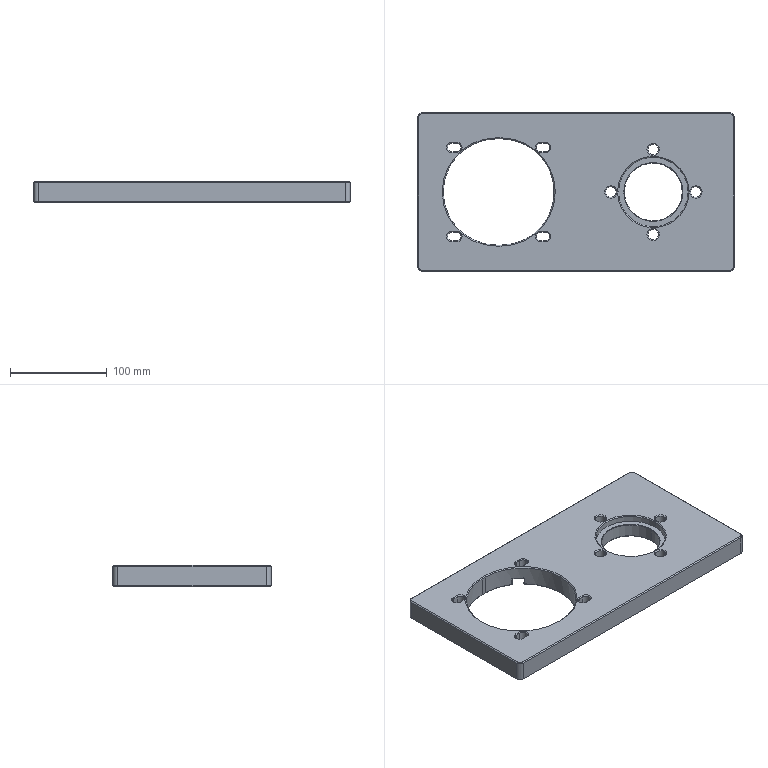NC program | NX | posted with a generic post | part box 328 x 164 x 22 mm
Lines 1 to 575 of 34171:
N10 G17 G21 G94 G90
(DRILLING , TOOL : ZXZ)
N12 T01 M6
N14 G54
N16 G17 G0 G90 X80. Y44. S5000 M3
N18 G43 Z30. H1
N20 G94 G81 G98 Z-1. F250. R3.
N22 Y0.
N24 X36.
N26 X80. Y-44.
N28 X124. Y0.
N30 G80
N32 G0 X124. Y0. Z30.
(DRILLING_COPY , TOOL : ZXZ)
N34 X-31.538 Y45.962
N36 G81 Z-1. F250. R3.
N38 X-123.462
N40 Y-45.962
N42 X-31.538
N44 G80
N46 G0 X-31.538 Y-45.962 Z30.
N48 M5
(DRILLING_COPY_COPY , TOOL : 11.0ZT)
N50 T11 M6
N52 G54
N54 G17 G0 G90 X80. Y44. S1200 M3
N56 G43 Z30. H11
N58 G94 G83 G98 Z-25.305 F250. Q2. R3.
N60 Y0.
N62 X36.
N64 X80. Y-44.
N66 X124. Y0.
N68 G80
N70 G0 X124. Y0. Z30.
N72 M5
(DRILLING_COPY_COPY_1 , TOOL : 6.8ZT)
N74 T16 M6
N76 G54
N78 G17 G0 G90 X-31.538 Y45.962 S2000 M3
N80 G43 Z30. H16
N82 G94 G83 G98 Z-24.043 F250. Q2. R3.
N84 X-123.462
N86 Y-45.962
N88 X-31.538
N90 G80
N92 G0 X-31.538 Y-45.962 Z30.
N94 M5
(HOLE_MILLING_COPY , TOOL : D26)
N96 T02 M6
N98 G54
N100 G17 G0 G90 X80. Y0. S1700 M3
N102 G43 Z30. H2
N104 Z0.5
N106 G94 G3 X85.713 Y-5.713 R5.712 F1000.
N108 X91.425 Y0. R5.712
N110 X91.425 Y0. Z0.2 I-11.425 J0. F2000.
N112 X91.425 Y0. Z-0.1 I-11.425 J0.
N114 X91.425 Y0. Z-0.4 I-11.425 J0.
N116 X91.425 Y0. Z-0.7 I-11.425 J0.
N118 X91.425 Y0. Z-1. I-11.425 J0.
N120 X91.425 Y0. Z-1.3 I-11.425 J0.
N122 X91.425 Y0. Z-1.6 I-11.425 J0.
N124 X91.425 Y0. Z-1.9 I-11.425 J0.
N126 X91.425 Y0. Z-2.2 I-11.425 J0.
N128 X91.425 Y0. Z-2.5 I-11.425 J0.
N130 X91.425 Y0. Z-2.8 I-11.425 J0.
N132 X91.425 Y0. Z-3.1 I-11.425 J0.
N134 X91.425 Y0. Z-3.4 I-11.425 J0.
N136 X91.425 Y0. Z-3.7 I-11.425 J0.
N138 X91.425 Y0. Z-4. I-11.425 J0.
N140 X91.425 Y0. Z-4.3 I-11.425 J0.
N142 X91.425 Y0. Z-4.6 I-11.425 J0.
N144 X91.425 Y0. Z-4.9 I-11.425 J0.
N146 X91.425 Y0. Z-5.2 I-11.425 J0.
N148 X91.425 Y0. Z-5.5 I-11.425 J0.
N150 X91.425 Y0. Z-5.8 I-11.425 J0.
N152 X91.425 Y0. Z-6.1 I-11.425 J0.
N154 X91.425 Y0. Z-6.4 I-11.425 J0.
N156 X91.425 Y0. Z-6.7 I-11.425 J0.
N158 X91.425 Y0. Z-7. I-11.425 J0.
N160 X80. Y11.425 R11.425
N162 X91.425 Y0. R-11.425
N164 X85.713 Y5.713 R5.712
N166 X80. Y0. R5.712
N168 G0 Z0.5
N170 G3 X91.425 Y-11.425 R11.425 F1000.
N172 X102.85 Y0. R11.425
N174 X102.85 Y0. Z0.2 I-22.85 J0. F2000.
N176 X102.85 Y0. Z-0.1 I-22.85 J0.
N178 X102.85 Y0. Z-0.4 I-22.85 J0.
N180 X102.85 Y0. Z-0.7 I-22.85 J0.
N182 X102.85 Y0. Z-1. I-22.85 J0.
N184 X102.85 Y0. Z-1.3 I-22.85 J0.
N186 X102.85 Y0. Z-1.6 I-22.85 J0.
N188 X102.85 Y0. Z-1.9 I-22.85 J0.
N190 X102.85 Y0. Z-2.2 I-22.85 J0.
N192 X102.85 Y0. Z-2.5 I-22.85 J0.
N194 X102.85 Y0. Z-2.8 I-22.85 J0.
N196 X102.85 Y0. Z-3.1 I-22.85 J0.
N198 X102.85 Y0. Z-3.4 I-22.85 J0.
N200 X102.85 Y0. Z-3.7 I-22.85 J0.
N202 X102.85 Y0. Z-4. I-22.85 J0.
N204 X102.85 Y0. Z-4.3 I-22.85 J0.
N206 X102.85 Y0. Z-4.6 I-22.85 J0.
N208 X102.85 Y0. Z-4.9 I-22.85 J0.
N210 X102.85 Y0. Z-5.2 I-22.85 J0.
N212 X102.85 Y0. Z-5.5 I-22.85 J0.
N214 X102.85 Y0. Z-5.8 I-22.85 J0.
N216 X102.85 Y0. Z-6.1 I-22.85 J0.
N218 X102.85 Y0. Z-6.4 I-22.85 J0.
N220 X102.85 Y0. Z-6.7 I-22.85 J0.
N222 X102.85 Y0. Z-7. I-22.85 J0.
N224 X80. Y22.85 R22.85
N226 X102.85 Y0. R-22.85
N228 X91.425 Y11.425 R11.425
N230 X80. Y0. R11.425
N232 G0 Z30.
(HOLE_MILLING_COPY_COPY , TOOL : D26)
N234 Z-6.5
N236 G3 X84.213 Y-4.213 R4.212 F1000.
N238 X88.425 Y0. R4.212
N240 X88.425 Y0. Z-6.8 I-8.425 J0. F2000.
N242 X88.425 Y0. Z-7.1 I-8.425 J0.
N244 X88.425 Y0. Z-7.4 I-8.425 J0.
N246 X88.425 Y0. Z-7.7 I-8.425 J0.
N248 X88.425 Y0. Z-8. I-8.425 J0.
N250 X88.425 Y0. Z-8.3 I-8.425 J0.
N252 X88.425 Y0. Z-8.6 I-8.425 J0.
N254 X88.425 Y0. Z-8.9 I-8.425 J0.
N256 X88.425 Y0. Z-9.2 I-8.425 J0.
N258 X88.425 Y0. Z-9.5 I-8.425 J0.
N260 X88.425 Y0. Z-9.8 I-8.425 J0.
N262 X88.425 Y0. Z-10.1 I-8.425 J0.
N264 X88.425 Y0. Z-10.4 I-8.425 J0.
N266 X88.425 Y0. Z-10.7 I-8.425 J0.
N268 X88.425 Y0. Z-11. I-8.425 J0.
N270 X88.425 Y0. Z-11.3 I-8.425 J0.
N272 X88.425 Y0. Z-11.6 I-8.425 J0.
N274 X88.425 Y0. Z-11.9 I-8.425 J0.
N276 X88.425 Y0. Z-12.2 I-8.425 J0.
N278 X88.425 Y0. Z-12.5 I-8.425 J0.
N280 X88.425 Y0. Z-12.8 I-8.425 J0.
N282 X88.425 Y0. Z-13.1 I-8.425 J0.
N284 X88.425 Y0. Z-13.4 I-8.425 J0.
N286 X88.425 Y0. Z-13.7 I-8.425 J0.
N288 X88.425 Y0. Z-14. I-8.425 J0.
N290 X88.425 Y0. Z-14.3 I-8.425 J0.
N292 X88.425 Y0. Z-14.6 I-8.425 J0.
N294 X88.425 Y0. Z-14.9 I-8.425 J0.
N296 X88.425 Y0. Z-15.2 I-8.425 J0.
N298 X88.425 Y0. Z-15.5 I-8.425 J0.
N300 X88.425 Y0. Z-15.8 I-8.425 J0.
N302 X88.425 Y0. Z-16.1 I-8.425 J0.
N304 X88.425 Y0. Z-16.4 I-8.425 J0.
N306 X88.425 Y0. Z-16.7 I-8.425 J0.
N308 X88.425 Y0. Z-17. I-8.425 J0.
N310 X88.425 Y0. Z-17.3 I-8.425 J0.
N312 X88.425 Y0. Z-17.6 I-8.425 J0.
N314 X88.425 Y0. Z-17.9 I-8.425 J0.
N316 X88.425 Y0. Z-18.2 I-8.425 J0.
N318 X88.425 Y0. Z-18.5 I-8.425 J0.
N320 X88.425 Y0. Z-18.8 I-8.425 J0.
N322 X88.425 Y0. Z-19.1 I-8.425 J0.
N324 X88.425 Y0. Z-19.4 I-8.425 J0.
N326 X88.425 Y0. Z-19.7 I-8.425 J0.
N328 X88.425 Y0. Z-20. I-8.425 J0.
N330 X88.425 Y0. Z-20.3 I-8.425 J0.
N332 X88.425 Y0. Z-20.6 I-8.425 J0.
N334 X88.425 Y0. Z-20.9 I-8.425 J0.
N336 X88.425 Y0. Z-21.2 I-8.425 J0.
N338 X88.425 Y0. Z-21.5 I-8.425 J0.
N340 X88.425 Y0. Z-21.8 I-8.425 J0.
N342 X88.425 Y0. Z-22.1 I-8.425 J0.
N344 X88.425 Y0. Z-22.4 I-8.425 J0.
N346 X88.425 Y0. Z-22.7 I-8.425 J0.
N348 X75.788 Y7.296 Z-22.8 R8.425
N350 X72.704 Y-4.213 R8.425
N352 X75.788 Y7.296 R-8.425
N354 X74.246 Y1.542 R4.212
N356 X80. Y0. R4.212
N358 G0 Z-6.5
N360 G3 X88.425 Y-8.425 R8.425 F1000.
N362 X96.85 Y0. R8.425
N364 X96.85 Y0. Z-6.8 I-16.85 J0. F2000.
N366 X96.85 Y0. Z-7.1 I-16.85 J0.
N368 X96.85 Y0. Z-7.4 I-16.85 J0.
N370 X96.85 Y0. Z-7.7 I-16.85 J0.
N372 X96.85 Y0. Z-8. I-16.85 J0.
N374 X96.85 Y0. Z-8.3 I-16.85 J0.
N376 X96.85 Y0. Z-8.6 I-16.85 J0.
N378 X96.85 Y0. Z-8.9 I-16.85 J0.
N380 X96.85 Y0. Z-9.2 I-16.85 J0.
N382 X96.85 Y0. Z-9.5 I-16.85 J0.
N384 X96.85 Y0. Z-9.8 I-16.85 J0.
N386 X96.85 Y0. Z-10.1 I-16.85 J0.
N388 X96.85 Y0. Z-10.4 I-16.85 J0.
N390 X96.85 Y0. Z-10.7 I-16.85 J0.
N392 X96.85 Y0. Z-11. I-16.85 J0.
N394 X96.85 Y0. Z-11.3 I-16.85 J0.
N396 X96.85 Y0. Z-11.6 I-16.85 J0.
N398 X96.85 Y0. Z-11.9 I-16.85 J0.
N400 X96.85 Y0. Z-12.2 I-16.85 J0.
N402 X96.85 Y0. Z-12.5 I-16.85 J0.
N404 X96.85 Y0. Z-12.8 I-16.85 J0.
N406 X96.85 Y0. Z-13.1 I-16.85 J0.
N408 X96.85 Y0. Z-13.4 I-16.85 J0.
N410 X96.85 Y0. Z-13.7 I-16.85 J0.
N412 X96.85 Y0. Z-14. I-16.85 J0.
N414 X96.85 Y0. Z-14.3 I-16.85 J0.
N416 X96.85 Y0. Z-14.6 I-16.85 J0.
N418 X96.85 Y0. Z-14.9 I-16.85 J0.
N420 X96.85 Y0. Z-15.2 I-16.85 J0.
N422 X96.85 Y0. Z-15.5 I-16.85 J0.
N424 X96.85 Y0. Z-15.8 I-16.85 J0.
N426 X96.85 Y0. Z-16.1 I-16.85 J0.
N428 X96.85 Y0. Z-16.4 I-16.85 J0.
N430 X96.85 Y0. Z-16.7 I-16.85 J0.
N432 X96.85 Y0. Z-17. I-16.85 J0.
N434 X96.85 Y0. Z-17.3 I-16.85 J0.
N436 X96.85 Y0. Z-17.6 I-16.85 J0.
N438 X96.85 Y0. Z-17.9 I-16.85 J0.
N440 X96.85 Y0. Z-18.2 I-16.85 J0.
N442 X96.85 Y0. Z-18.5 I-16.85 J0.
N444 X96.85 Y0. Z-18.8 I-16.85 J0.
N446 X96.85 Y0. Z-19.1 I-16.85 J0.
N448 X96.85 Y0. Z-19.4 I-16.85 J0.
N450 X96.85 Y0. Z-19.7 I-16.85 J0.
N452 X96.85 Y0. Z-20. I-16.85 J0.
N454 X96.85 Y0. Z-20.3 I-16.85 J0.
N456 X96.85 Y0. Z-20.6 I-16.85 J0.
N458 X96.85 Y0. Z-20.9 I-16.85 J0.
N460 X96.85 Y0. Z-21.2 I-16.85 J0.
N462 X96.85 Y0. Z-21.5 I-16.85 J0.
N464 X96.85 Y0. Z-21.8 I-16.85 J0.
N466 X96.85 Y0. Z-22.1 I-16.85 J0.
N468 X96.85 Y0. Z-22.4 I-16.85 J0.
N470 X96.85 Y0. Z-22.7 I-16.85 J0.
N472 X71.575 Y14.593 Z-22.8 R16.85
N474 X65.407 Y-8.425 R16.85
N476 X71.575 Y14.593 R-16.85
N478 X68.491 Y3.084 R8.425
N480 X80. Y0. R8.425
N482 G0 Z30.
(HOLE_MILLING_COPY_COPY_COPY , TOOL : D26)
N484 X-82.5
N486 Z-0.5
N488 G3 X-77.269 Y-5.231 R5.231 F1000.
N490 X-72.038 Y0. R5.231
N492 X-72.038 Y0. Z-0.8 I-10.462 J0. F2000.
N494 X-72.038 Y0. Z-1.1 I-10.462 J0.
N496 X-72.038 Y0. Z-1.4 I-10.462 J0.
N498 X-72.038 Y0. Z-1.7 I-10.462 J0.
N500 X-72.038 Y0. Z-2. I-10.462 J0.
N502 X-72.038 Y0. Z-2.3 I-10.462 J0.
N504 X-72.038 Y0. Z-2.6 I-10.462 J0.
N506 X-72.038 Y0. Z-2.9 I-10.462 J0.
N508 X-72.038 Y0. Z-3.2 I-10.462 J0.
N510 X-72.038 Y0. Z-3.5 I-10.462 J0.
N512 X-72.038 Y0. Z-3.8 I-10.462 J0.
N514 X-72.038 Y0. Z-4.1 I-10.462 J0.
N516 X-72.038 Y0. Z-4.4 I-10.462 J0.
N518 X-72.038 Y0. Z-4.7 I-10.462 J0.
N520 X-72.038 Y0. Z-5. I-10.462 J0.
N522 X-72.038 Y0. Z-5.3 I-10.462 J0.
N524 X-72.038 Y0. Z-5.6 I-10.462 J0.
N526 X-72.038 Y0. Z-5.9 I-10.462 J0.
N528 X-72.038 Y0. Z-6.2 I-10.462 J0.
N530 X-72.038 Y0. Z-6.5 I-10.462 J0.
N532 X-72.038 Y0. Z-6.8 I-10.462 J0.
N534 X-72.038 Y0. Z-7.1 I-10.462 J0.
N536 X-72.038 Y0. Z-7.4 I-10.462 J0.
N538 X-72.038 Y0. Z-7.7 I-10.462 J0.
N540 X-72.038 Y0. Z-8. I-10.462 J0.
N542 X-72.038 Y0. Z-8.3 I-10.462 J0.
N544 X-72.038 Y0. Z-8.6 I-10.462 J0.
N546 X-72.038 Y0. Z-8.9 I-10.462 J0.
N548 X-72.038 Y0. Z-9.2 I-10.462 J0.
N550 X-72.038 Y0. Z-9.5 I-10.462 J0.
N552 X-72.038 Y0. Z-9.8 I-10.462 J0.
N554 X-72.038 Y0. Z-10.1 I-10.462 J0.
N556 X-72.038 Y0. Z-10.4 I-10.462 J0.
N558 X-72.038 Y0. Z-10.7 I-10.462 J0.
N560 X-72.038 Y0. Z-11. I-10.462 J0.
N562 X-72.038 Y0. Z-11.3 I-10.462 J0.
N564 X-72.038 Y0. Z-11.6 I-10.462 J0.
N566 X-72.038 Y0. Z-11.9 I-10.462 J0.
N568 X-72.038 Y0. Z-12.2 I-10.462 J0.
N570 X-72.038 Y0. Z-12.5 I-10.462 J0.
N572 X-72.038 Y0. Z-12.8 I-10.462 J0.
N574 X-72.038 Y0. Z-13.1 I-10.462 J0.
N576 X-72.038 Y0. Z-13.4 I-10.462 J0.
N578 X-72.038 Y0. Z-13.7 I-10.462 J0.
N580 X-72.038 Y0. Z-14. I-10.462 J0.
N582 X-72.038 Y0. Z-14.3 I-10.462 J0.
N584 X-72.038 Y0. Z-14.6 I-10.462 J0.
N586 X-72.038 Y0. Z-14.9 I-10.462 J0.
N588 X-72.038 Y0. Z-15.2 I-10.462 J0.
N590 X-72.038 Y0. Z-15.5 I-10.462 J0.
N592 X-72.038 Y0. Z-15.8 I-10.462 J0.
N594 X-72.038 Y0. Z-16.1 I-10.462 J0.
N596 X-72.038 Y0. Z-16.4 I-10.462 J0.
N598 X-72.038 Y0. Z-16.7 I-10.462 J0.
N600 X-72.038 Y0. Z-17. I-10.462 J0.
N602 X-72.038 Y0. Z-17.3 I-10.462 J0.
N604 X-72.038 Y0. Z-17.6 I-10.462 J0.
N606 X-72.038 Y0. Z-17.9 I-10.462 J0.
N608 X-72.038 Y0. Z-18.2 I-10.462 J0.
N610 X-72.038 Y0. Z-18.5 I-10.462 J0.
N612 X-72.038 Y0. Z-18.8 I-10.462 J0.
N614 X-72.038 Y0. Z-19.1 I-10.462 J0.
N616 X-72.038 Y0. Z-19.4 I-10.462 J0.
N618 X-72.038 Y0. Z-19.7 I-10.462 J0.
N620 X-72.038 Y0. Z-20. I-10.462 J0.
N622 X-72.038 Y0. Z-20.3 I-10.462 J0.
N624 X-72.038 Y0. Z-20.6 I-10.462 J0.
N626 X-72.038 Y0. Z-20.9 I-10.462 J0.
N628 X-72.038 Y0. Z-21.2 I-10.462 J0.
N630 X-72.038 Y0. Z-21.5 I-10.462 J0.
N632 X-72.038 Y0. Z-21.8 I-10.462 J0.
N634 X-82.5 Y10.463 R10.462
N636 X-72.038 Y0. R-10.462
N638 X-77.269 Y5.231 R5.231
N640 X-82.5 Y0. R5.231
N642 G0 Z-0.5
N644 G3 X-72.038 Y-10.463 R10.462 F1000.
N646 X-61.575 Y0. R10.462
N648 X-61.575 Y0. Z-0.8 I-20.925 J0. F2000.
N650 X-61.575 Y0. Z-1.1 I-20.925 J0.
N652 X-61.575 Y0. Z-1.4 I-20.925 J0.
N654 X-61.575 Y0. Z-1.7 I-20.925 J0.
N656 X-61.575 Y0. Z-2. I-20.925 J0.
N658 X-61.575 Y0. Z-2.3 I-20.925 J0.
N660 X-61.575 Y0. Z-2.6 I-20.925 J0.
N662 X-61.575 Y0. Z-2.9 I-20.925 J0.
N664 X-61.575 Y0. Z-3.2 I-20.925 J0.
N666 X-61.575 Y0. Z-3.5 I-20.925 J0.
N668 X-61.575 Y0. Z-3.8 I-20.925 J0.
N670 X-61.575 Y0. Z-4.1 I-20.925 J0.
N672 X-61.575 Y0. Z-4.4 I-20.925 J0.
N674 X-61.575 Y0. Z-4.7 I-20.925 J0.
N676 X-61.575 Y0. Z-5. I-20.925 J0.
N678 X-61.575 Y0. Z-5.3 I-20.925 J0.
N680 X-61.575 Y0. Z-5.6 I-20.925 J0.
N682 X-61.575 Y0. Z-5.9 I-20.925 J0.
N684 X-61.575 Y0. Z-6.2 I-20.925 J0.
N686 X-61.575 Y0. Z-6.5 I-20.925 J0.
N688 X-61.575 Y0. Z-6.8 I-20.925 J0.
N690 X-61.575 Y0. Z-7.1 I-20.925 J0.
N692 X-61.575 Y0. Z-7.4 I-20.925 J0.
N694 X-61.575 Y0. Z-7.7 I-20.925 J0.
N696 X-61.575 Y0. Z-8. I-20.925 J0.
N698 X-61.575 Y0. Z-8.3 I-20.925 J0.
N700 X-61.575 Y0. Z-8.6 I-20.925 J0.
N702 X-61.575 Y0. Z-8.9 I-20.925 J0.
N704 X-61.575 Y0. Z-9.2 I-20.925 J0.
N706 X-61.575 Y0. Z-9.5 I-20.925 J0.
N708 X-61.575 Y0. Z-9.8 I-20.925 J0.
N710 X-61.575 Y0. Z-10.1 I-20.925 J0.
N712 X-61.575 Y0. Z-10.4 I-20.925 J0.
N714 X-61.575 Y0. Z-10.7 I-20.925 J0.
N716 X-61.575 Y0. Z-11. I-20.925 J0.
N718 X-61.575 Y0. Z-11.3 I-20.925 J0.
N720 X-61.575 Y0. Z-11.6 I-20.925 J0.
N722 X-61.575 Y0. Z-11.9 I-20.925 J0.
N724 X-61.575 Y0. Z-12.2 I-20.925 J0.
N726 X-61.575 Y0. Z-12.5 I-20.925 J0.
N728 X-61.575 Y0. Z-12.8 I-20.925 J0.
N730 X-61.575 Y0. Z-13.1 I-20.925 J0.
N732 X-61.575 Y0. Z-13.4 I-20.925 J0.
N734 X-61.575 Y0. Z-13.7 I-20.925 J0.
N736 X-61.575 Y0. Z-14. I-20.925 J0.
N738 X-61.575 Y0. Z-14.3 I-20.925 J0.
N740 X-61.575 Y0. Z-14.6 I-20.925 J0.
N742 X-61.575 Y0. Z-14.9 I-20.925 J0.
N744 X-61.575 Y0. Z-15.2 I-20.925 J0.
N746 X-61.575 Y0. Z-15.5 I-20.925 J0.
N748 X-61.575 Y0. Z-15.8 I-20.925 J0.
N750 X-61.575 Y0. Z-16.1 I-20.925 J0.
N752 X-61.575 Y0. Z-16.4 I-20.925 J0.
N754 X-61.575 Y0. Z-16.7 I-20.925 J0.
N756 X-61.575 Y0. Z-17. I-20.925 J0.
N758 X-61.575 Y0. Z-17.3 I-20.925 J0.
N760 X-61.575 Y0. Z-17.6 I-20.925 J0.
N762 X-61.575 Y0. Z-17.9 I-20.925 J0.
N764 X-61.575 Y0. Z-18.2 I-20.925 J0.
N766 X-61.575 Y0. Z-18.5 I-20.925 J0.
N768 X-61.575 Y0. Z-18.8 I-20.925 J0.
N770 X-61.575 Y0. Z-19.1 I-20.925 J0.
N772 X-61.575 Y0. Z-19.4 I-20.925 J0.
N774 X-61.575 Y0. Z-19.7 I-20.925 J0.
N776 X-61.575 Y0. Z-20. I-20.925 J0.
N778 X-61.575 Y0. Z-20.3 I-20.925 J0.
N780 X-61.575 Y0. Z-20.6 I-20.925 J0.
N782 X-61.575 Y0. Z-20.9 I-20.925 J0.
N784 X-61.575 Y0. Z-21.2 I-20.925 J0.
N786 X-61.575 Y0. Z-21.5 I-20.925 J0.
N788 X-61.575 Y0. Z-21.8 I-20.925 J0.
N790 X-82.5 Y20.925 R20.925
N792 X-61.575 Y0. R-20.925
N794 X-72.038 Y10.463 R10.462
N796 X-82.5 Y0. R10.462
N798 G0 Z-0.5
N800 G3 X-66.806 Y-15.694 R15.694 F1000.
N802 X-51.113 Y0. R15.694
N804 X-51.113 Y0. Z-0.8 I-31.387 J0. F2000.
N806 X-51.113 Y0. Z-1.1 I-31.387 J0.
N808 X-51.113 Y0. Z-1.4 I-31.387 J0.
N810 X-51.113 Y0. Z-1.7 I-31.387 J0.
N812 X-51.113 Y0. Z-2. I-31.387 J0.
N814 X-51.113 Y0. Z-2.3 I-31.387 J0.
N816 X-51.113 Y0. Z-2.6 I-31.387 J0.
N818 X-51.113 Y0. Z-2.9 I-31.387 J0.
N820 X-51.113 Y0. Z-3.2 I-31.387 J0.
N822 X-51.113 Y0. Z-3.5 I-31.387 J0.
N824 X-51.113 Y0. Z-3.8 I-31.387 J0.
N826 X-51.113 Y0. Z-4.1 I-31.387 J0.
N828 X-51.113 Y0. Z-4.4 I-31.387 J0.
N830 X-51.113 Y0. Z-4.7 I-31.387 J0.
N832 X-51.113 Y0. Z-5. I-31.387 J0.
N834 X-51.113 Y0. Z-5.3 I-31.387 J0.
N836 X-51.113 Y0. Z-5.6 I-31.387 J0.
N838 X-51.113 Y0. Z-5.9 I-31.387 J0.
N840 X-51.113 Y0. Z-6.2 I-31.387 J0.
N842 X-51.113 Y0. Z-6.5 I-31.387 J0.
N844 X-51.113 Y0. Z-6.8 I-31.387 J0.
N846 X-51.113 Y0. Z-7.1 I-31.387 J0.
N848 X-51.113 Y0. Z-7.4 I-31.387 J0.
N850 X-51.113 Y0. Z-7.7 I-31.387 J0.
N852 X-51.113 Y0. Z-8. I-31.387 J0.
N854 X-51.113 Y0. Z-8.3 I-31.387 J0.
N856 X-51.113 Y0. Z-8.6 I-31.387 J0.
N858 X-51.113 Y0. Z-8.9 I-31.387 J0.
N860 X-51.113 Y0. Z-9.2 I-31.387 J0.
N862 X-51.113 Y0. Z-9.5 I-31.387 J0.
N864 X-51.113 Y0. Z-9.8 I-31.387 J0.
N866 X-51.113 Y0. Z-10.1 I-31.387 J0.
N868 X-51.113 Y0. Z-10.4 I-31.387 J0.
N870 X-51.113 Y0. Z-10.7 I-31.387 J0.
N872 X-51.113 Y0. Z-11. I-31.387 J0.
N874 X-51.113 Y0. Z-11.3 I-31.387 J0.
N876 X-51.113 Y0. Z-11.6 I-31.387 J0.
N878 X-51.113 Y0. Z-11.9 I-31.387 J0.
N880 X-51.113 Y0. Z-12.2 I-31.387 J0.
N882 X-51.113 Y0. Z-12.5 I-31.387 J0.
N884 X-51.113 Y0. Z-12.8 I-31.387 J0.
N886 X-51.113 Y0. Z-13.1 I-31.387 J0.
N888 X-51.113 Y0. Z-13.4 I-31.387 J0.
N890 X-51.113 Y0. Z-13.7 I-31.387 J0.
N892 X-51.113 Y0. Z-14. I-31.387 J0.
N894 X-51.113 Y0. Z-14.3 I-31.387 J0.
N896 X-51.113 Y0. Z-14.6 I-31.387 J0.
N898 X-51.113 Y0. Z-14.9 I-31.387 J0.
N900 X-51.113 Y0. Z-15.2 I-31.387 J0.
N902 X-51.113 Y0. Z-15.5 I-31.387 J0.
N904 X-51.113 Y0. Z-15.8 I-31.387 J0.
N906 X-51.113 Y0. Z-16.1 I-31.387 J0.
N908 X-51.113 Y0. Z-16.4 I-31.387 J0.
N910 X-51.113 Y0. Z-16.7 I-31.387 J0.
N912 X-51.113 Y0. Z-17. I-31.387 J0.
N914 X-51.113 Y0. Z-17.3 I-31.387 J0.
N916 X-51.113 Y0. Z-17.6 I-31.387 J0.
N918 X-51.113 Y0. Z-17.9 I-31.387 J0.
N920 X-51.113 Y0. Z-18.2 I-31.387 J0.
N922 X-51.113 Y0. Z-18.5 I-31.387 J0.
N924 X-51.113 Y0. Z-18.8 I-31.387 J0.
N926 X-51.113 Y0. Z-19.1 I-31.387 J0.
N928 X-51.113 Y0. Z-19.4 I-31.387 J0.
N930 X-51.113 Y0. Z-19.7 I-31.387 J0.
N932 X-51.113 Y0. Z-20. I-31.387 J0.
N934 X-51.113 Y0. Z-20.3 I-31.387 J0.
N936 X-51.113 Y0. Z-20.6 I-31.387 J0.
N938 X-51.113 Y0. Z-20.9 I-31.387 J0.
N940 X-51.113 Y0. Z-21.2 I-31.387 J0.
N942 X-51.113 Y0. Z-21.5 I-31.387 J0.
N944 X-51.113 Y0. Z-21.8 I-31.387 J0.
N946 X-82.5 Y31.388 R31.387
N948 X-51.113 Y0. R-31.387
N950 X-66.806 Y15.694 R15.694
N952 X-82.5 Y0. R15.694
N954 G0 Z-0.5
N956 G3 X-61.575 Y-20.925 R20.925 F1000.
N958 X-40.65 Y0. R20.925
N960 X-40.65 Y0. Z-0.8 I-41.85 J0. F2000.
N962 X-40.65 Y0. Z-1.1 I-41.85 J0.
N964 X-40.65 Y0. Z-1.4 I-41.85 J0.
N966 X-40.65 Y0. Z-1.7 I-41.85 J0.
N968 X-40.65 Y0. Z-2. I-41.85 J0.
N970 X-40.65 Y0. Z-2.3 I-41.85 J0.
N972 X-40.65 Y0. Z-2.6 I-41.85 J0.
N974 X-40.65 Y0. Z-2.9 I-41.85 J0.
N976 X-40.65 Y0. Z-3.2 I-41.85 J0.
N978 X-40.65 Y0. Z-3.5 I-41.85 J0.
N980 X-40.65 Y0. Z-3.8 I-41.85 J0.
N982 X-40.65 Y0. Z-4.1 I-41.85 J0.
N984 X-40.65 Y0. Z-4.4 I-41.85 J0.
N986 X-40.65 Y0. Z-4.7 I-41.85 J0.
N988 X-40.65 Y0. Z-5. I-41.85 J0.
N990 X-40.65 Y0. Z-5.3 I-41.85 J0.
N992 X-40.65 Y0. Z-5.6 I-41.85 J0.
N994 X-40.65 Y0. Z-5.9 I-41.85 J0.
N996 X-40.65 Y0. Z-6.2 I-41.85 J0.
N998 X-40.65 Y0. Z-6.5 I-41.85 J0.
N1000 X-40.65 Y0. Z-6.8 I-41.85 J0.
N1002 X-40.65 Y0. Z-7.1 I-41.85 J0.
N1004 X-40.65 Y0. Z-7.4 I-41.85 J0.
N1006 X-40.65 Y0. Z-7.7 I-41.85 J0.
N1008 X-40.65 Y0. Z-8. I-41.85 J0.
N1010 X-40.65 Y0. Z-8.3 I-41.85 J0.
N1012 X-40.65 Y0. Z-8.6 I-41.85 J0.
N1014 X-40.65 Y0. Z-8.9 I-41.85 J0.
N1016 X-40.65 Y0. Z-9.2 I-41.85 J0.
N1018 X-40.65 Y0. Z-9.5 I-41.85 J0.
N1020 X-40.65 Y0. Z-9.8 I-41.85 J0.
N1022 X-40.65 Y0. Z-10.1 I-41.85 J0.
N1024 X-40.65 Y0. Z-10.4 I-41.85 J0.
N1026 X-40.65 Y0. Z-10.7 I-41.85 J0.
N1028 X-40.65 Y0. Z-11. I-41.85 J0.
N1030 X-40.65 Y0. Z-11.3 I-41.85 J0.
N1032 X-40.65 Y0. Z-11.6 I-41.85 J0.
N1034 X-40.65 Y0. Z-11.9 I-41.85 J0.
N1036 X-40.65 Y0. Z-12.2 I-41.85 J0.
N1038 X-40.65 Y0. Z-12.5 I-41.85 J0.
N1040 X-40.65 Y0. Z-12.8 I-41.85 J0.
N1042 X-40.65 Y0. Z-13.1 I-41.85 J0.
N1044 X-40.65 Y0. Z-13.4 I-41.85 J0.
N1046 X-40.65 Y0. Z-13.7 I-41.85 J0.
N1048 X-40.65 Y0. Z-14. I-41.85 J0.
N1050 X-40.65 Y0. Z-14.3 I-41.85 J0.
N1052 X-40.65 Y0. Z-14.6 I-41.85 J0.
N1054 X-40.65 Y0. Z-14.9 I-41.85 J0.
N1056 X-40.65 Y0. Z-15.2 I-41.85 J0.
N1058 X-40.65 Y0. Z-15.5 I-41.85 J0.
N1060 X-40.65 Y0. Z-15.8 I-41.85 J0.
N1062 X-40.65 Y0. Z-16.1 I-41.85 J0.
N1064 X-40.65 Y0. Z-16.4 I-41.85 J0.
N1066 X-40.65 Y0. Z-16.7 I-41.85 J0.
N1068 X-40.65 Y0. Z-17. I-41.85 J0.
N1070 X-40.65 Y0. Z-17.3 I-41.85 J0.
N1072 X-40.65 Y0. Z-17.6 I-41.85 J0.
N1074 X-40.65 Y0. Z-17.9 I-41.85 J0.
N1076 X-40.65 Y0. Z-18.2 I-41.85 J0.
N1078 X-40.65 Y0. Z-18.5 I-41.85 J0.
N1080 X-40.65 Y0. Z-18.8 I-41.85 J0.
N1082 X-40.65 Y0. Z-19.1 I-41.85 J0.
N1084 X-40.65 Y0. Z-19.4 I-41.85 J0.
N1086 X-40.65 Y0. Z-19.7 I-41.85 J0.
N1088 X-40.65 Y0. Z-20. I-41.85 J0.
N1090 X-40.65 Y0. Z-20.3 I-41.85 J0.
N1092 X-40.65 Y0. Z-20.6 I-41.85 J0.
N1094 X-40.65 Y0. Z-20.9 I-41.85 J0.
N1096 X-40.65 Y0. Z-21.2 I-41.85 J0.
N1098 X-40.65 Y0. Z-21.5 I-41.85 J0.
N1100 X-40.65 Y0. Z-21.8 I-41.85 J0.
N1102 X-82.5 Y41.85 R41.85
N1104 X-40.65 Y0. R-41.85
N1106 X-61.575 Y20.925 R20.925
N1108 X-82.5 Y0. R20.925
N1110 G0 Z30.
N1112 M5